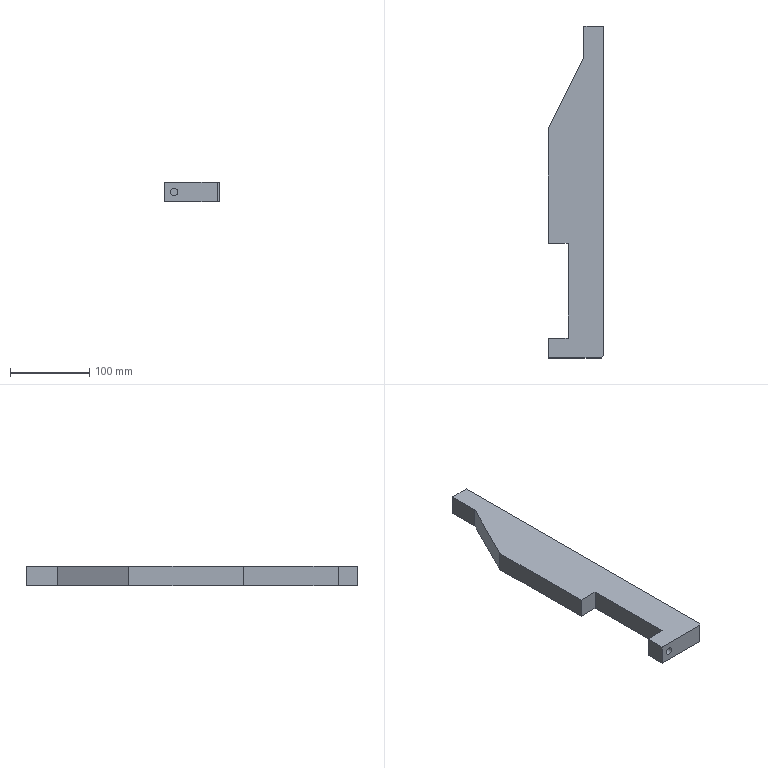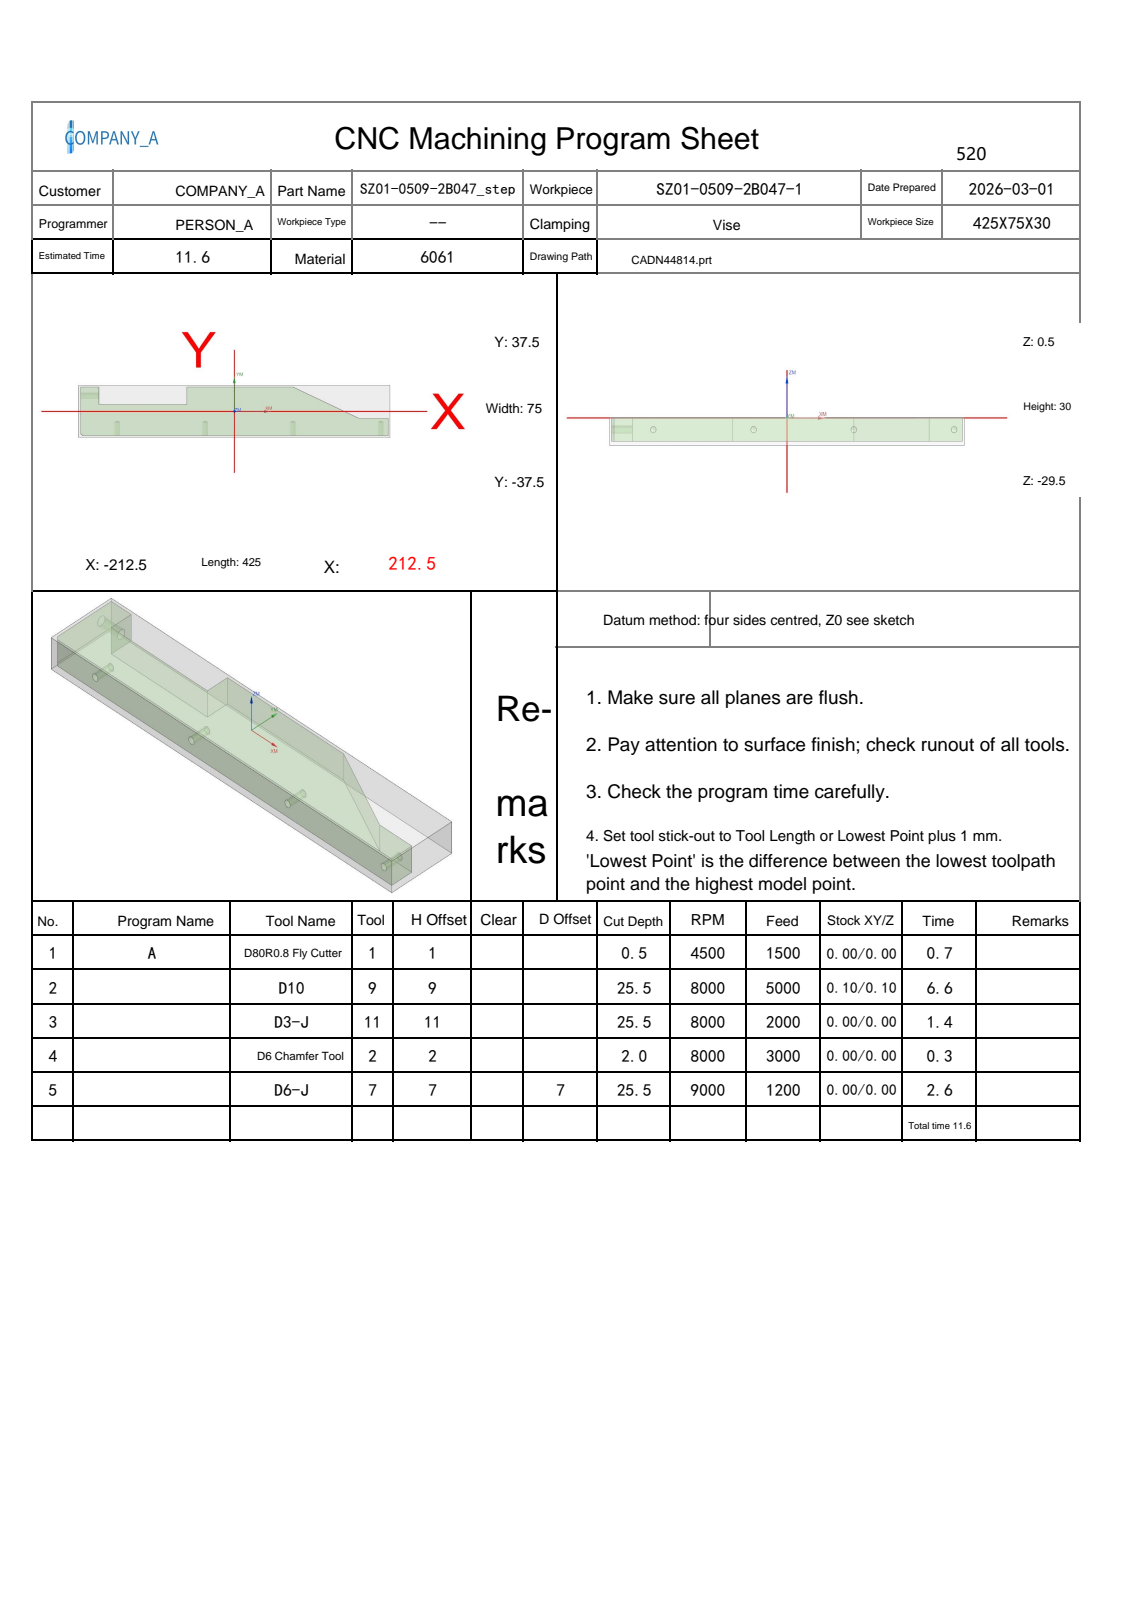NC program | NX | posted by the shop | part box 70 x 420 x 25 mm
Lines 34 to 885 of 10764:
N2 T09 M06
(D10  D=10. R=0. H=09 ce=0.10 di=0.10)
G00 G90 G54 X-211.098 Y48.981 M03 S8000
G43 H09 Z50.
M08
Z-10.5
G01 X-211.079 Y48.882 Z-11.125 F5000.
X-211.06 Y48.784 Z-11.372
X-211.042 Y48.686 Z-11.554
X-211.023 Y48.588 Z-11.7
X-211.004 Y48.489 Z-11.823
X-210.986 Y48.391 Z-11.928
X-210.967 Y48.293 Z-12.02
X-210.948 Y48.195 Z-12.1
X-210.93 Y48.096 Z-12.17
X-210.911 Y47.998 Z-12.232
X-210.892 Y47.9 Z-12.286
X-210.873 Y47.802 Z-12.333
X-210.855 Y47.703 Z-12.374
X-210.836 Y47.605 Z-12.408
X-210.817 Y47.507 Z-12.436
X-210.799 Y47.409 Z-12.46
X-210.78 Y47.31 Z-12.477
X-210.761 Y47.212 Z-12.49
X-210.743 Y47.114 Z-12.497
X-210.724 Y47.016 Z-12.5
X-210.322 Y44.901
G03 X-210.063 Y44.55 I.505 J.101
X-207.898 Y44.057 I2.979 J8.086
X-203.397 Y43.804 I4.918 J47.355
G01 X-198.079 Y43.754
X-192.762 Y43.75
X210.278 Y43.745
X210.332
G02 X213.413 Y43.193 I0.0 J-8.878
X216.7 Y40.387 I-2.504 J-6.262
X218.094 Y36.737 I-9.76 J-5.821
X218.61 Y32.292 I-27.885 J-5.484
X218.744 Y25.632 I-164.482 J-6.66
X218.743 Y25.014 I-164.616 J0.0
G01 X218.744 Y-35.286
Y-35.333
G02 X218.219 Y-38.345 I-8.894 J0.0
X215.371 Y-41.709 I-6.294 J2.441
X211.722 Y-43.097 I-5.817 J9.801
X207.277 Y-43.611 I-5.483 J27.985
X200.682 Y-43.744 I-6.595 J163.023
X200.079 Y-43.743 I0.0 J163.156
G01 X-210.301
X-210.348 Y-43.744
G02 X-213.434 Y-43.184 I0.0 J8.798
X-216.693 Y-40.395 I2.531 J6.255
X-218.076 Y-36.819 I9.68 J5.8
X-218.605 Y-32.376 I27.224 J5.494
X-218.745 Y-25.631 I162.596 J6.745
X-218.743 Y-24.858 I162.735 J0.0
G01 X-218.746 Y35.202
Y35.281
G02 X-218.275 Y38.192 I9.232 J0.0
X-215.412 Y41.682 I6.328 J-2.272
X-212.197 Y42.838 I4.466 J-7.372
X-208.856 Y43.082 I3.341 J-22.715
X-208.449 Y43.079 I0.0 J-22.959
G03 X-194.641 Y42.948 I13.808 J732.57
X-192.841 Y42.951 I0.0 J732.7
G01 X208.339 Y42.945
X208.433
G02 X211.028 Y42.602 I0.0 J-10.003
X215.115 Y39.67 I-2.294 J-7.51
X216.96 Y35.704 I-9.667 J-6.912
X217.695 Y31.129 I-24.183 J-6.229
X217.92 Y24.975 I-92.838 J-6.481
G01 X217.949 Y20.215
Y15.455
X217.943 Y-33.357
X217.944 Y-33.452
G02 X217.572 Y-36.123 I-9.783 J0.0
X214.653 Y-40.126 I-7.495 J2.4
X210.683 Y-41.966 I-6.904 J9.693
X205.948 Y-42.709 I-6.306 J24.717
X199.393 Y-42.926 I-6.673 J102.243
G01 X194.833 Y-42.95
X190.273 Y-42.949
X-208.417 Y-42.942
X-208.483
G02 X-211.18 Y-42.555 I0.0 J9.582
X-215.172 Y-39.589 I2.477 J7.503
X-216.99 Y-35.595 I9.889 J6.911
X-217.716 Y-30.857 I25.281 J6.3
X-217.927 Y-24.302 I105.092 J6.664
G01 X-217.95 Y-19.782
X-217.949 Y-15.262
X-217.942 Y33.417
Y33.491
G02 X-217.531 Y36.256 I9.508 J0.0
X-214.455 Y40.134 I6.941 J-2.347
X-210.756 Y41.599 I5.902 J-9.499
X-206.309 Y42.097 I5.084 J-25.281
X-201.368 Y42.17 I4.941 J-168.306
X-199.75 Y42.162 I0.0 J-168.379
G01 X-191.482 Y42.151
X206.338 Y42.147
X206.525 Y42.148
G02 X209.349 Y41.797 I0.0 J-11.517
X214.093 Y38.446 I-2.386 J-8.411
X216.07 Y34.175 I-10.63 J-7.515
X216.873 Y29.207 I-26.289 J-6.796
X217.122 Y22.253 I-101.87 J-7.137
G01 X217.149 Y17.573
Y12.893
X217.142 Y-31.567
Y-31.664
G02 X216.632 Y-34.873 I-10.358 J0.0
X213.375 Y-39.145 I-8.263 J2.922
X209.315 Y-41.033 I-7.473 J10.761
X204.671 Y-41.834 I-6.622 J24.55
X198.198 Y-42.111 I-6.94 J86.445
G01 X192.678 Y-42.148
X187.158 Y-42.149
X-206.502 Y-42.143
X-206.625 Y-42.144
G02 X-209.735 Y-41.678 I0.0 J10.635
X-214.156 Y-38.356 I2.809 J8.34
X-216.096 Y-34.08 I10.872 J7.51
X-216.881 Y-29.109 I26.852 J6.788
X-217.123 Y-22.154 I104.98 J7.142
G01 X-217.149 Y-17.475
Y-12.795
X-217.143 Y31.505
Y31.63
G02 X-216.761 Y34.43 I10.439 J0.0
X-213.525 Y38.779 I7.78 J-2.41
G01 X-212.732 Y39.277
X-212.474 Y39.457
X-212.193 Y39.597
G02 X-207.834 Y40.878 I6.502 J-14.066
X-203.293 Y41.269 I5.33 J-35.332
X-196.45 Y41.356 I6.843 J-267.272
X-194.734 Y41.351 I0.0 J-267.359
G01 X204.766 Y41.344
X204.851
G02 X208.165 Y40.894 I0.0 J-12.42
X213.248 Y37.135 I-2.769 J-9.061
X215.231 Y32.695 I-11.702 J-7.89
X216.059 Y27.486 I-28.446 J-7.191
X216.317 Y20.532 I-103.929 J-7.335
G01 X216.348 Y15.333
Y10.133
X216.341 Y-29.767
X216.342 Y-29.818
G02 X215.899 Y-33.168 I-12.901 J0.0
X215.123 Y-35.013 I-9.07 J2.732
G01 X214.926 Y-36.32
X214.417 Y-37.55
X213.606 Y-38.606
X212.55 Y-39.417
X211.32 Y-39.926
X208.1 Y-40.508
G02 X199.979 Y-41.238 I-9.465 J59.704
X190.704 Y-41.351 I-9.275 J380.949
X188.94 Y-41.347 I0.0 J381.062
G01 X-204.56 Y-41.344
X-204.739 Y-41.345
G02 X-208.2 Y-40.889 I0.0 J13.358
X-212.77 Y-37.798 I2.596 J8.761
X-214.665 Y-34.466 I9.16 J7.415
X-215.841 Y-29.577 I19.995 J7.396
X-216.245 Y-24.155 I50.116 J6.458
X-216.353 Y-15.09 I380.886 J9.065
X-216.347 Y-13.116 I380.994 J0.0
G01 X-216.342 Y29.744
Y29.834
G02 X-215.893 Y33.062 I11.813 J0.0
X-215.158 Y34.745 I8.337 J-2.637
G01 X-214.926 Y36.32
X-214.417 Y37.55
X-213.606 Y38.606
X-212.55 Y39.417
X-211.32 Y39.926
G02 X-207.985 Y40.188 I3.92 J-28.537
X-195.137 Y40.568 I12.847 J-216.987
X-192.234 Y40.549 I0.0 J-217.367
G01 X203.586 Y40.53
X203.726 Y40.531
G02 X210.819 Y37.793 I0.0 J-10.56
X214.395 Y31.352 I-9.432 J-9.45
X215.428 Y22.711 I-39.034 J-9.046
X215.556 Y10.949 I-538.454 J-11.762
X215.548 Y7.992 I-538.582 J0.0
G01 X215.523 Y-28.707
G02 X215.1 Y-31.802 I-15.852 J.589
G01 X215.079 Y-35.16
X215.08 Y-9.746
G02 X214.893 Y-1.17 I196.509 J8.577
X214.908 Y1.281 I196.696 J0.0
G03 X214.931 Y7.234 I-782.365 J5.952
X214.788 Y22.2 I-782.387 J0.0
X213.77 Y30.682 I-39.156 J-.396
X210.244 Y36.877 I-12.083 J-2.775
X204.158 Y39.5 I-7.341 J-8.662
X197.059 Y39.906 I-7.099 J-61.922
X196.014 Y39.897 I0.0 J-62.328
G01 X81.257 Y39.933
X80.001 Y40.1
X-65.249 Y40.08
G02 X-74.105 Y39.893 I-8.856 J209.56
X-76.761 Y39.91 I0.0 J209.747
G01 X-183.712 Y39.93
X-184.998 Y40.1
X-209.638
G02 X-210.138 Y40.6 I0.0 J.5
X-209.906 Y41.022 I.5 J0.0
G01 X-209.148 Y41.502
X-207.483 Y42.557 Z-12.4
X-207.151 Y42.767
X-207.091 Y42.8
X-207.027 Y42.824
X-206.961 Y42.839
X-206.894 Y42.845
X-185.653 Y43.292
X-185.566 Y43.286
X-185.481 Y43.266
X-185.402 Y43.231
X-185.329 Y43.182
X-185.266 Y43.122
X-185.215 Y43.052
X-185.176 Y42.974
X-185.027 Y42.59
X-184.31 Y40.752 Z-12.5
X-184.079 Y40.176
G03 X-183.712 Y39.93 I.439 J.259
X-180.141 Y39.292 I3.782 J10.844
X-170.849 Y39.093 I9.292 J217.517
X-168.122 Y39.11 I0.0 J217.715
G01 X-70.492 Y39.136
X-70.323 Y39.135
G03 X-67.856 Y39.219 I0.0 J36.232
G02 X-66.32 Y39.926 I4.077 J-6.837
G01 X-64.998 Y40.1
X-66.32 Y39.926
X-67.55 Y39.417
G02 X-69.04 Y38.871 I-1.684 J2.29
X-75.014 Y38.49 I-5.974 J46.74
X-75.685 Y38.495 I0.0 J47.12
G01 X-173.209 Y38.484
G02 X-174.324 Y38.474 I-1.116 J66.91
X-181.303 Y38.839 I0.0 J66.919
X-181.882 Y38.981 I.759 J4.365
G03 X-183.411 Y39.815 I-2.713 J-3.155
G02 X-181.755 Y38.883 I-1.263 J-4.183
G03 X-178.605 Y38.039 I3.777 J7.792
X-170.778 Y37.677 I7.827 J84.423
X-169.701 Y37.684 I0.0 J84.785
G01 X-76.335 Y37.695
G03 X-75.655 Y37.69 I.68 J43.925
X-69.676 Y38.099 I0.0 J43.93
X-68.754 Y38.413 I-.094 J1.786
G02 X-67.781 Y39.239 I3.269 J-2.864
G03 X-68.859 Y38.293 I2.343 J-3.757
G02 X-71.8 Y37.416 I-3.508 J6.39
X-79.465 Y37.032 I-7.665 J76.38
X-80.701 Y37.042 I0.0 J76.763
G01 X-170.316 Y37.052
G02 X-171.191 Y37.046 I-.875 J62.731
X-178.77 Y37.506 I0.0 J62.737
X-180.98 Y38.107 I1.186 J8.714
G03 X-181.775 Y38.898 I-3.184 J-2.405
G02 X-180.971 Y38.062 I-1.558 J-2.3
G03 X-178.205 Y36.921 I3.677 J4.991
X-170.776 Y36.29 I7.429 J43.448
G01 X-170.517 Y36.291
G03 X-161.369 Y36.227 I9.148 J655.618
X-159.402 Y36.23 I0.0 J655.681
G01 X-80.165 Y36.25
G03 X-79.337 Y36.245 I.828 J61.013
X-72.076 Y36.678 I0.0 J61.019
X-69.513 Y37.437 I-.707 J7.094
G01 X-68.776 Y38.386
G02 X-69.774 Y37.191 I-5.218 J3.349
X-73.292 Y36.064 I-4.341 J7.491
X-81.063 Y35.611 I-7.77 J66.531
X-81.761 Y35.615 I0.0 J66.983
G01 X-166.803 Y35.607
G02 X-167.823 Y35.601 I-1.02 J80.96
X-176.372 Y36.054 I0.0 J80.967
X-180.373 Y37.23 I.934 J10.566
G01 X-181.07 Y38.185
G02 X-180.343 Y37.131 I-9.646 J-7.434
G03 X-177.614 Y35.766 I3.99 J4.569
X-170.671 Y34.927 I7.376 J31.891
X-159.882 Y34.785 I10.788 J407.675
X-157.641 Y34.791 I0.0 J407.817
G01 X-82.094 Y34.818
G03 X-81.359 Y34.813 I.735 J59.663
X-73.412 Y35.345 I0.0 J59.667
X-69.896 Y36.591 I-1.005 J8.414
X-69.417 Y37.55 I-2.259 J1.729
G02 X-69.938 Y36.478 I-3.576 J1.075
X-72.827 Y35.049 I-4.113 J4.682
X-79.876 Y34.261 I-7.324 J33.571
X-90.205 Y34.151 I-10.33 J485.363
G01 X-90.762
X-165.509 Y34.179
G02 X-166.266 Y34.175 I-.757 J73.052
X-175.262 Y34.731 I0.0 J73.055
X-179.594 Y36.111 I1.295 J11.558
X-180.205 Y36.637 I1.194 J2.003
G01 X-180.511 Y37.376
G03 X-178.623 Y35.219 I3.191 J.888
X-173.561 Y33.858 I6.49 J14.046
X-163.55 Y33.359 I10.011 J100.22
X-162.339 Y33.367 I0.0 J100.719
G01 X-84.727 Y33.374
G03 X-83.922 Y33.37 I.805 J73.9
X-75.176 Y33.889 I0.0 J73.904
X-70.746 Y35.282 I-1.267 J11.769
X-69.961 Y36.059 I-.664 J1.456
G02 X-69.743 Y36.763 I2.046 J-.247
G03 X-69.991 Y35.902 I2.233 J-1.11
G02 X-71.857 Y34.387 I-3.303 J2.162
X-77.458 Y33.089 I-6.739 J16.342
X-87.76 Y32.702 I-10.302 J136.791
X-89.648 Y32.715 I0.0 J137.179
G01 X-162.561 Y32.732
G02 X-163.491 Y32.727 I-.93 J93.423
X-173.27 Y33.24 I0.0 J93.427
X-178.563 Y34.706 I1.487 J15.659
X-179.99 Y35.869 I1.733 J3.584
G03 X-180.196 Y36.616 I-3.612 J-.595
G02 X-180.002 Y35.823 I-2.206 J-.96
G03 X-178.141 Y34.059 I3.513 J1.842
X-172.652 Y32.498 I7.148 J14.699
X-162.576 Y31.938 I10.076 J90.42
X-161.923 Y31.94 I0.0 J90.979
G01 X-152.042 Y31.911
X-87.122 Y31.931
G03 X-86.14 Y31.925 I.982 J85.132
X-76.514 Y32.471 I0.0 J85.138
X-71.36 Y34.038 I-1.451 J14.032
X-70.087 Y35.192 I-1.533 J2.969
G01 X-69.962 Y36.052
G02 X-70.186 Y34.913 I-3.389 J.076
X-72.555 Y33.066 I-4.186 J2.926
X-78.73 Y31.67 I-7.503 J18.835
X-89.489 Y31.264 I-10.758 J142.224
X-91.33 Y31.275 I0.0 J142.63
G01 X-161.115 Y31.296
G02 X-161.955 Y31.292 I-.84 J93.375
X-172.288 Y31.866 I0.0 J93.379
X-178.062 Y33.518 I1.723 J16.939
X-179.901 Y35.127 I2.093 J4.247
G01 X-180.023 Y35.93
G03 X-178.677 Y33.492 I2.93 J.027
X-173.934 Y31.513 I6.894 J9.851
X-164.788 Y30.593 I9.66 J50.083
X-152.946 Y30.468 I11.843 J563.542
X-151.401 Y30.471 I0.0 J563.667
G01 X-88.486 Y30.495
G03 X-87.682 Y30.491 I.804 J88.608
X-77.625 Y31.064 I0.0 J88.612
X-71.941 Y32.738 I-1.695 J16.24
X-70.141 Y34.345 I-2.185 J4.258
X-70.068 Y35.24 I-16.842 J1.82
G01 X-70.109 Y34.358
G02 X-71.851 Y32.427 I-3.629 J1.521
X-77.292 Y30.589 I-7.394 J12.92
X-87.369 Y29.88 I-10.077 J71.286
G01 X-87.628 Y29.881
X-96.12 Y29.83
X-158.723 Y29.851
G02 X-159.717 Y29.847 I-.994 J110.54
X-170.739 Y30.397 I0.0 J110.545
X-177.278 Y32.114 I1.865 J20.415
X-179.829 Y34.277 I2.357 J5.368
X-179.922 Y35.06 I3.256 J.783
G01 X-179.921 Y35.157
X-179.925 Y34.985
G03 X-179.79 Y33.986 I3.766 J0.0
X-177.383 Y31.653 I4.75 J2.493
X-171.213 Y29.778 I8.397 J16.545
X-160.33 Y29.082 I10.883 J84.643
G01 X-160.141
X-149.721 Y29.031
X-90.719 Y29.05
G03 X-89.688 Y29.045 I1.031 J101.913
X-78.899 Y29.618 I0.0 J101.918
X-72.575 Y31.358 I-1.893 J19.242
X-70.139 Y33.486 I-2.383 J5.186
X-70.092 Y34.178 I-5.094 J.693
X-70.1 Y34.455 I-5.141 J0.0
G02 X-70.08 Y34.085 I-3.496 J-.37
X-70.172 Y33.288 I-3.516 J0.0
X-72.417 Y31.038 I-4.537 J2.281
X-78.58 Y29.12 I-8.268 J15.71
X-89.251 Y28.435 I-10.671 J82.739
G01 X-89.54
X-99.162 Y28.391
X-156.964 Y28.41
G02 X-157.901 Y28.407 I-.937 J122.954
X-169.408 Y28.946 I0.0 J122.958
X-176.562 Y30.707 I2.049 J23.733
X-179.639 Y33.099 I2.796 J6.775
X-179.9 Y33.664 I2.468 J1.481
G01 Y34.464
G03 X-179.923 Y34.071 I3.349 J-.392
X-179.73 Y32.948 I3.372 J0.0
X-177.02 Y30.386 I5.406 J3.003
X-170.411 Y28.384 I9.08 J18.069
X-158.906 Y27.643 I11.504 J88.865
G01 X-158.702
X-147.961 Y27.591
X-92.239 Y27.611
G03 X-91.246 Y27.606 I.993 J109.609
X-79.946 Y28.19 I0.0 J109.613
X-73.165 Y29.97 I-2.144 J21.98
X-70.182 Y32.443 I-2.699 J6.289
X-70.077 Y33.214 I-2.759 J.771
X-70.1 Y33.578 I-2.864 J0.0
G02 X-70.081 Y33.181 I-4.248 J-.397
X-70.166 Y32.335 I-4.266 J0.0
X-72.356 Y29.99 I-4.721 J2.214
X-78.392 Y27.883 I-8.571 J14.856
X-88.938 Y27.033 I-10.852 J68.819
X-98.681 Y26.951 I-10.074 J618.993
G01 X-155.523 Y26.971
G02 X-156.407 Y26.968 I-.884 J129.811
X-168.377 Y27.521 I0.0 J129.814
X-175.972 Y29.33 I2.269 J26.368
X-179.567 Y32.031 I3.034 J7.781
X-179.9 Y32.717 I2.217 J1.5
G01 Y33.597
G03 X-179.925 Y33.165 I3.775 J-.432
X-179.738 Y31.988 I3.8 J0.0
X-176.99 Y29.271 I5.702 J3.018
X-170.259 Y27.083 I9.542 J17.909
X-158.68 Y26.228 I11.791 J80.863
X-148.177 Y26.148 I10.502 J688.641
X-145.882 Y26.152 I0.0 J688.721
G01 X-93.362 Y26.174
G03 X-92.531 Y26.171 I.831 J114.018
X-80.85 Y26.771 I0.0 J114.021
X-73.59 Y28.635 I-2.346 J24.2
X-70.263 Y31.289 I-2.993 J7.165
X-70.1 Y31.689 I-3.854 J1.807
G01 Y32.649
G02 X-70.082 Y32.219 I-5.042 J-.43
X-70.161 Y31.326 I-5.061 J0.0
X-72.269 Y28.937 I-4.831 J2.139
X-78.474 Y26.602 I-9.022 J14.56
X-89.357 Y25.616 I-11.384 J65.094
X-100.522 Y25.512 I-11.442 J632.823
G01 X-154.955 Y25.539
G02 X-155.708 Y25.536 I-.752 J120.323
X-168.169 Y26.183 I0.0 J120.326
X-175.852 Y28.136 I2.637 J26.461
X-179.56 Y31. I3.33 J8.142
X-179.9 Y31.704 I2.378 J1.584
G01 Y32.584
G03 X-179.924 Y32.15 I3.98 J-.434
X-179.754 Y30.997 I4.004 J0.0
X-177.082 Y28.206 I5.832 J2.908
X-170.257 Y25.806 I9.959 J17.418
X-158.891 Y24.824 I12.043 J73.141
X-147.241 Y24.712 I11.972 J640.042
G01 X-95.038 Y24.732
G03 X-94.04 Y24.728 I.998 J122.943
X-81.722 Y25.347 I0.0 J122.947
X-73.95 Y27.308 I-2.507 J26.315
X-70.378 Y30.045 I-3.315 J8.026
X-70.1 Y30.627 I-1.748 J1.192
G01 Y31.667
G02 X-70.08 Y31.2 I-5.499 J-.467
X-70.161 Y30.258 I-5.518 J0.0
X-72.332 Y27.761 I-5.059 J2.206
X-78.546 Y25.319 I-9.394 J14.777
X-89.619 Y24.205 I-11.842 J62.086
X-102.006 Y24.069 I-12.387 J565.576
X-103.961 Y24.072 I0.0 J565.711
G01 X-153.041 Y24.094
G02 X-153.89 Y24.091 I-.849 J137.364
X-166.85 Y24.704 I0.0 J137.367
X-175.202 Y26.681 I2.708 J30.074
X-179.374 Y29.669 I3.628 J9.473
X-179.9 Y30.664 I2.377 J1.893
G01 Y31.624
G03 X-179.924 Y31.133 I5.091 J-.491
X-179.826 Y30.137 I5.115 J0.0
X-177.544 Y27.381 I5.475 J2.21
X-171.101 Y24.714 I10.023 J15.097
X-160.083 Y23.465 I12.319 J59.44
X-146.829 Y23.265 I13.254 J438.575
X-144.201 Y23.273 I0.0 J438.775
G01 X-96.239 Y23.293
G03 X-95.298 Y23.29 I.941 J129.197
X-82.591 Y23.916 I0.0 J129.2
X-74.388 Y25.924 I-2.692 J28.751
X-70.445 Y28.845 I-3.512 J8.862
X-70.1 Y29.534 I-1.682 J1.274
G01 Y30.574
G02 X-70.076 Y30.074 I-5.148 J-.5
X-70.154 Y29.177 I-5.172 J0.0
X-72.334 Y26.606 I-5.184 J2.187
X-78.818 Y23.987 I-9.877 J15.116
X-89.881 Y22.795 I-12.173 J61.075
X-102.258 Y22.629 I-12.377 J460.009
X-104.041 Y22.632 I0.0 J460.175
G01 X-151.921 Y22.656
G02 X-152.823 Y22.653 I-.902 J138.143
X-166.355 Y23.317 I0.0 J138.146
X-174.957 Y25.386 I2.95 J31.187
X-179.293 Y28.462 I3.9 J10.091
X-179.9 Y29.58 I2.579 J2.124
G01 Y30.54
G03 X-179.922 Y30.074 I4.812 J-.466
X-179.773 Y28.882 I4.834 J0.0
X-177.197 Y25.982 I6.031 J2.764
X-170.135 Y23.224 I10.754 J17.114
X-158.529 Y22.008 I12.879 J66.903
X-145.115 Y21.826 I13.414 J496.498
X-142.601 Y21.833 I0.0 J496.679
G01 X-97.677 Y21.852
G03 X-96.752 Y21.849 I.925 J141.717
X-83.759 Y22.446 I0.0 J141.72
X-75.012 Y24.449 I-2.792 J32.3
X-70.682 Y27.398 I-3.847 J10.299
X-70.1 Y28.407 I-1.989 J1.821
G01 Y29.527
G02 X-70.082 Y29.034 I-6.784 J-.493
X-70.154 Y28.048 I-6.802 J0.0
X-72.261 Y25.489 I-5.231 J2.159
X-78.668 Y22.746 I-10.115 J14.778
X-89.677 Y21.408 I-12.536 J57.162
X-102.824 Y21.185 I-13.147 J387.358
X-105.402 Y21.193 I0.0 J387.581
G01 X-151.434 Y21.223
G02 X-152.129 Y21.221 I-.695 J133.742
X-166.013 Y21.944 I0.0 J133.743
X-174.987 Y24.194 I3.135 J31.522
X-179.218 Y27.237 I4.258 J10.383
X-179.9 Y28.456 I3.022 J2.49
G01 Y29.496
G03 X-179.925 Y28.995 I5.081 J-.501
X-179.77 Y27.746 I5.106 J0.0
X-177.265 Y24.855 I6.139 J2.788
X-170.363 Y21.995 I10.96 J16.695
X-158.892 Y20.626 I13.198 J61.855
X-144.348 Y20.38 I14.544 J428.921
X-140.922 Y20.393 I0.0 J429.168
G01 X-98.559 Y20.415
G03 X-97.606 Y20.411 I.953 J139.586
X-84.024 Y21.074 I0.0 J139.589
X-75.042 Y23.213 I-3.035 J32.664
X-70.711 Y26.206 I-4.106 J10.573
X-70.1 Y27.249 I-2.156 J1.964
G01 Y28.369
G02 X-70.08 Y27.869 I-6.184 J-.499
X-70.16 Y26.877 I-6.204 J0.0
X-72.338 Y24.243 I-5.44 J2.279
X-78.788 Y21.437 I-10.453 J15.218
X-90.093 Y19.995 I-13.009 J56.949
X-103.238 Y19.748 I-13.145 J349.222
X-105.241 Y19.754 I0.0 J349.469
G01 X-150.235 Y19.783
G02 X-150.774 Y19.782 I-.539 J145.336
X-164.847 Y20.465 I0.0 J145.337
X-174.2 Y22.632 I3.28 J35.423
X-179.013 Y25.832 I4.443 J11.901
X-179.9 Y27.313 I3.196 J2.921
G01 Y28.353
G03 X-179.923 Y27.855 I5.306 J-.499
X-179.779 Y26.624 I5.33 J0.0
X-177.339 Y23.719 I6.164 J2.699
X-170.264 Y20.688 I11.306 J16.62
X-158.323 Y19.206 I13.771 J62.101
X-143.63 Y18.941 I14.693 J407.097
X-140.362 Y18.954 I0.0 J407.362
G01 X-99.599 Y18.976
G03 X-98.626 Y18.973 I.973 J143.049
X-84.586 Y19.663 I0.0 J143.052
X-75.233 Y21.898 I-3.183 J34.018
X-70.656 Y25.101 I-4.16 J10.816
X-70.1 Y26.082 I-2.104 J1.84
G01 Y27.202
G02 X-70.083 Y26.716 I-6.804 J-.486
X-70.156 Y25.719 I-6.822 J0.0
X-72.311 Y23.059 I-5.483 J2.24
X-78.973 Y20.105 I-10.834 J15.442
X-90.506 Y18.582 I-13.449 J57.399
X-105.295 Y18.297 I-14.788 J383.663
X-108.921 Y18.314 I0.0 J383.948
G01 X-148.085 Y18.335
G02 X-149.054 Y18.332 I-.969 J163.326
X-163.83 Y19.002 I0.0 J163.329
X-173.755 Y21.212 I3.337 J38.379
X-178.873 Y24.497 I4.643 J12.861
X-179.9 Y26.146 I3.195 J3.135
G01 Y27.186
G03 X-179.922 Y26.676 I5.865 J-.51
X-179.813 Y25.548 I5.888 J0.0
X-177.42 Y22.575 I6.131 J2.484
X-170.551 Y19.476 I11.442 J16.202
X-158.609 Y17.829 I14.139 J58.396
X-142.906 Y17.496 I15.703 J370.492
X-139.242 Y17.514 I0.0 J370.825
G01 X-99.768 Y17.544
G03 X-99.09 Y17.543 I.678 J136.467
X-84.694 Y18.304 I0.0 J136.469
X-75.3 Y20.624 I-3.512 J34.397
X-70.71 Y23.84 I-4.393 J11.153
X-70.1 Y24.895 I-2.264 J2.014
G01 Y26.015
G02 X-70.082 Y25.525 I-6.588 J-.49
X-70.158 Y24.526 I-6.607 J0.0
X-72.334 Y21.827 I-5.586 J2.277
X-79.014 Y18.805 I-11.099 J15.642
X-90.532 Y17.189 I-13.79 J56.445
X-105.521 Y16.859 I-14.989 J339.436
X-108.842 Y16.875 I0.0 J339.767
G01 X-147.283 Y16.897
G02 X-148.13 Y16.895 I-.847 J166.255
X-163.193 Y17.579 I0.0 J166.257
X-173.24 Y19.758 I3.573 J40.729
X-178.665 Y23.078 I4.859 J14.03
X-179.9 Y24.961 I3.397 J3.575
G01 Y26.001
G03 X-179.923 Y25.501 I5.42 J-.5
X-179.783 Y24.274 I5.443 J0.0
X-177.292 Y21.262 I6.42 J2.775
X-170.303 Y18.12 I11.78 J16.857
X-158.352 Y16.425 I14.451 J58.903
X-142.734 Y16.062 I15.619 J336.331
X-139.396 Y16.079 I0.0 J336.693
G01 X-102.152 Y16.096
G03 X-100.99 Y16.092 I1.161 J160.823
X-86.237 Y16.77 I0.0 J160.827
X-76.224 Y18.984 I-3.481 J39.492
X-71.041 Y22.245 I-4.638 J13.123
X-70.1 Y23.692 I-2.609 J2.725
G01 Y24.892
G02 X-70.08 Y24.366 I-7.056 J-.527
X-70.158 Y23.322 I-7.076 J0.0
X-72.353 Y20.585 I-5.683 J2.31
X-79.052 Y17.501 I-11.349 J15.837
X-91.123 Y15.778 I-14.079 J55.498
X-105.007 Y15.433 I-13.884 J279.212
X-107.088 Y15.441 I0.0 J279.557
G01 X-146.248 Y15.46
G02 X-147.208 Y15.457 I-.96 J166.927
X-163.168 Y16.222 I0.0 J166.93
X-173.287 Y18.513 I3.836 J40.434
X-178.727 Y21.938 I5.017 J14.004
X-179.9 Y23.77 I3.503 J3.535
G01 Y24.81
G03 X-179.923 Y24.309 I5.458 J-.501
X-179.781 Y23.07 I5.481 J0.0
X-177.271 Y20.02 I6.531 J2.817
X-170.253 Y16.812 I12.021 J17.016
X-159.187 Y15.1 I14.387 J56.377
G01 X-90.359 Y15.113
G03 X-77.664 Y17.19 I-1.34 J48.03
X-71.626 Y20.439 I-4.857 J16.259
X-70.106 Y22.442 I-3.31 J4.09
G01 X-70.1 Y23.675
G02 X-70.081 Y23.154 I-7.358 J-.521
X-70.155 Y22.112 I-7.377 J0.0
X-72.369 Y19.335 I-5.783 J2.34
X-79.081 Y16.199 I-11.551 J15.969
X-84.274 Y15.1 I-12.453 J46.022
G01 X-90.754
G03 X-87.232 Y15.078 I3.522 J282.658
X-81.565 Y15.135 I0.0 J282.68
X-72.236 Y18.689 I-1.873 J18.938
X-70.12 Y21.149 I-4.154 J5.714
G01 X-70.1 Y22.453
G02 X-70.081 Y21.927 I-7.243 J-.526
X-70.156 Y20.884 I-7.262 J0.0
X-72.325 Y18.131 I-5.771 J2.314
X-78.851 Y15.1 I-10.481 J14.029
G01 X-82.131
X-77.702 Y15.128
G03 X-70.698 Y18.982 I-1.63 J11.252
X-70.1 Y20.034 I-2.262 J1.983
G01 Y21.234
G02 X-70.08 Y20.705 I-7.178 J-.529
X-70.156 Y19.662 I-7.197 J0.0
X-72.336 Y16.929 I-5.619 J2.244
X-75.881 Y15.1 I-6.918 J9.062
G01 X-78.121
G03 X-77.037 Y15.079 I1.084 J27.596
X-75.043 Y15.151 I0.0 J27.617
X-70.153 Y18.65 I-1.517 J7.288
X-70.079 Y19.509 I-4.991 J.859
X-70.1 Y19.965 I-5.064 J0.0
G02 X-70.081 Y19.473 I-6.235 J-.492
X-70.161 Y18.475 I-6.254 J0.0
X-72.63 Y15.71 I-5.175 J2.137
X-73.941 Y15.1 I-3.763 J6.372
G01 X-75.541
G03 X-74.797 Y15.081 I.744 J14.586
X-73.322 Y15.156 I0.0 J14.605
X-70.122 Y17.683 I-1.226 J4.841
G01 X-70.1 Y18.832
G02 X-70.079 Y18.365 I-5.198 J-.467
X-70.165 Y17.419 I-5.219 J0.0
X-72.627 Y15.1 I-3.811 J1.579
G01 X-73.747
G03 X-73.226 Y15.081 I.521 J7.127
X-72.091 Y15.172 I0.0 J7.146
X-70.116 Y16.851 I-.945 J3.112
G01 X-70.1 Y17.743
G02 X-70.08 Y17.373 I-3.495 J-.37
X-70.172 Y16.575 I-3.514 J0.0
X-71.748 Y15.1 I-2.378 J.961
G01 X-72.468
G03 X-72.105 Y15.077 I.362 J2.788
X-71.042 Y15.286 I0.0 J2.811
X-70.1 Y16.329 I-.658 J1.54
G01 Y16.889
G02 X-70.076 Y16.605 I-1.669 J-.284
X-70.292 Y15.778 I-1.693 J0.0
X-71.46 Y15.083 I-1.168 J.634
X-71.671 Y15.1 I0.0 J1.329
G03 X-71.403 Y15.076 I.268 J1.471
X-70.144 Y15.765 I0.0 J1.495
X-70.1 Y16.264 I-4.771 J.674
G02 X-70.077 Y16.055 I-.938 J-.21
X-71.038 Y15.094 I-.961 J0.0
G01 X-71.146 Y15.1
G03 X-70.947 Y15.078 I.199 J.901
X-70.125 Y15.582 I0.0 J.923
G01 X-70.1 Y15.864
G03 X-70.65 Y16.414 I-.55 J0.0
X-71.152 Y16.089 I0.0 J-.55
X-71.294 Y15.608 I.868 J-.518
X-70.746 Y15.1 I.549 J.043
G01 X-70.711 Y15.099
G03 X-70.112 Y15.647 I0.0 J.601
G01 X-70.102 Y15.744
G03 X-70.257 Y16.108 I-.506 J0.0
G01 X-71.125 Y16.936
X-72.555 Y18.293 Z-12.4
X-72.624 Y18.336
X-72.698 Y18.367
X-72.776 Y18.386
X-72.856 Y18.392
X-156.442 Y17.845
X-156.529 Y17.837
X-156.613 Y17.814
X-156.692 Y17.776
X-156.763 Y17.726
X-156.824 Y17.664
X-156.899 Y17.573
X-158.159 Y16.056 Z-12.5
X-158.853 Y15.228
G02 X-159.187 Y15.1 I-.344 J.399
X-160.899 Y15.075 I-1.712 J58.614
X-164.833 Y15.207 I0.0 J58.639
X-175.353 Y18.208 I2.733 J29.514
X-179.416 Y21.589 I4.991 J10.13
X-179.9 Y22.56 I3.389 J2.297
G01 Y23.68
G03 X-179.925 Y23.144 I5.777 J-.536
X-179.779 Y21.853 I5.802 J0.0
X-177.306 Y18.811 I6.573 J2.816
X-170.462 Y15.592 I11.925 J16.476
G01 X-168.497 Y15.1
X-163.217
X-169.702 Y15.127
G02 X-178.42 Y19.173 I2.014 J15.751
X-179.9 Y21.342 I3.672 J4.096
G01 Y22.462
G03 X-179.925 Y21.925 I5.772 J-.538
X-179.778 Y20.627 I5.797 J0.0
X-177.2 Y17.496 I6.658 J2.854
X-172.42 Y15.1 I9.356 J12.701
G01 X-169.22
G02 X-170.676 Y15.075 I-1.457 J43.063
X-173.157 Y15.147 I0.0 J43.088
X-179.481 Y19.25 I2.03 J10.053
X-179.9 Y20.127 I3.551 J2.236
G01 Y21.247
G03 X-179.923 Y20.688 I6.727 J-.558
X-179.834 Y19.595 I6.75 J0.0
X-177.526 Y16.58 I5.945 J2.16
X-174.85 Y15.1 I5.778 J7.288
G01 X-172.69
X-175.227 Y15.126
G02 X-179.877 Y18.838 I1.513 J6.664
G01 X-179.9 Y19.99
G03 X-179.923 Y19.488 I5.406 J-.502
X-179.783 Y18.262 I5.429 J0.0
X-176.522 Y15.1 I5.297 J2.2
G01 X-175.002
G02 X-175.696 Y15.077 I-.694 J10.565
X-176.897 Y15.146 I0.0 J10.587
X-179.885 Y17.788 I1.399 J4.593
G01 X-179.9 Y18.837
G03 X-179.919 Y18.379 I5.433 J-.458
X-179.819 Y17.338 I5.452 J0.0
X-177.718 Y15.108 I3.602 J1.288
G01 X-176.555 Y15.1
G02 X-177.054 Y15.079 I-.499 J5.923
X-178.043 Y15.162 I0.0 J5.944
X-179.9 Y17.002 I.921 J2.787
G01 Y17.722
G03 X-179.923 Y17.353 I2.944 J-.368
X-179.732 Y16.307 I2.967 J0.0
X-178.453 Y15.1 I1.975 J.812
G01 X-177.733
G02 X-178.066 Y15.081 I-.333 J2.965
X-178.804 Y15.174 I0.0 J2.984
X-179.9 Y16.354 I.701 J1.75
G01 Y16.914
G03 X-179.925 Y16.617 I1.748 J-.297
X-179.268 Y15.239 I1.773 J0.0
X-178.664 Y15.082 I.604 J1.081
X-178.455 Y15.1 I0.0 J1.238
G02 X-178.704 Y15.075 I-.25 J1.234
X-179.894 Y15.922 I0.0 J1.259
G01 X-179.9 Y16.276
G03 X-179.924 Y16.055 I.984 J-.221
X-179.239 Y15.1 I1.009 J0.0
G01 X-178.999
X-179.149 Y15.085
G02 X-179.831 Y15.492 I0.0 J.776
X-179.895 Y15.748 I.487 J.256
X-179.345 Y16.298 I.55 J0.0
X-178.927 Y16.106 I0.0 J-.55
X-178.721 Y15.661 I-.378 J-.445
X-178.874 Y15.268 I-.583 J0.0
X-179.267 Y15.105 I-.393 J.393
G01 X-179.374 Y15.116
G02 X-179.921 Y15.776 I.124 J.66
G01 X-179.9 Y15.944
G02 X-179.724 Y16.325 I.513 J-.006
G01 X-178.938 Y16.995
X-177.438 Y18.275 Z-12.4
X-176.939 Y18.701
X-176.878 Y18.762
X-176.829 Y18.833
X-176.793 Y18.912
X-176.77 Y18.995
X-176.763 Y19.081
Y37.312
X-176.77 Y37.528
X-176.789 Y37.744
X-176.822 Y37.959
X-176.867 Y38.171
X-176.926 Y38.379
X-176.996 Y38.584
X-177.079 Y38.785
X-177.174 Y38.98